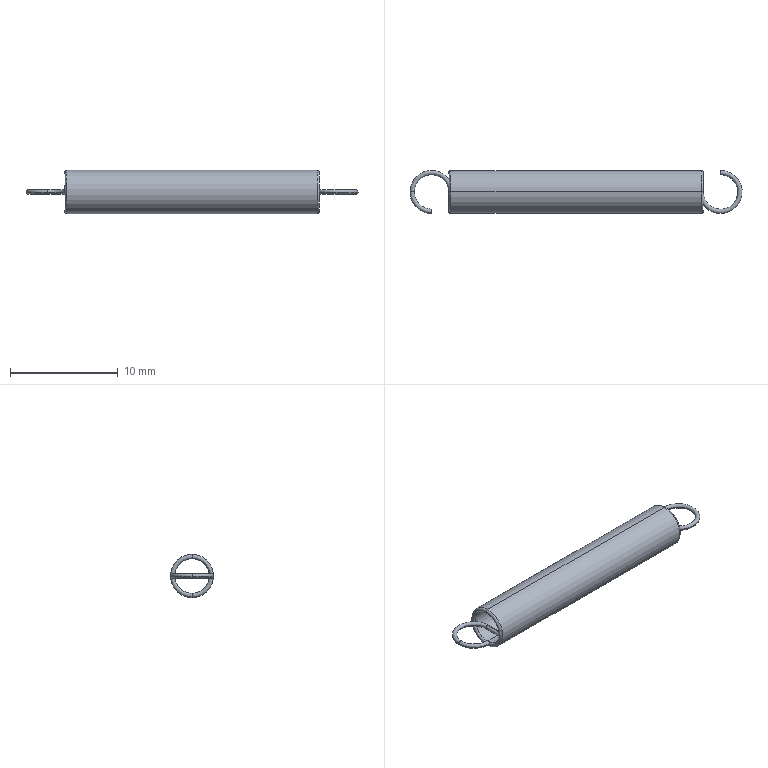Part | SolidWorks | features Revolution 5, RefAxis 1 | 1 solid | 20 faces | box 30.8 x 4 x 4 mm | volume 108.92 mm3 | torus 10 | cylinder 8 | plane 2 | commonest cylinder face diameters 0.4 x4 3.2 x2 4 x2
STEP:
#1=CARTESIAN_POINT('',(-0.4,0.,0.));
#2=VERTEX_POINT('',#1);
#3=CARTESIAN_POINT('',(0.,0.,0.));
#4=VERTEX_POINT('',#3);
#5=CARTESIAN_POINT('',(-0.2,0.,0.));
#6=DIRECTION('',(0.,-1.,0.));
#7=DIRECTION('',(0.,0.,-1.));
#8=AXIS2_PLACEMENT_3D('',#5,#6,#7);
#9=CIRCLE('',#8,0.2);
#10=EDGE_CURVE('',#2,#4,#9,.T.);
#11=ORIENTED_EDGE('',*,*,#10,.F.);
#12=CARTESIAN_POINT('',(3.6,0.,0.));
#13=VERTEX_POINT('',#12);
#14=CARTESIAN_POINT('',(1.6,0.,0.));
#15=DIRECTION('',(0.,0.,-1.));
#16=DIRECTION('',(-1.,0.,0.));
#17=AXIS2_PLACEMENT_3D('',#14,#15,#16);
#18=CIRCLE('',#17,2.);
#19=EDGE_CURVE('',#2,#13,#18,.T.);
#20=ORIENTED_EDGE('',*,*,#19,.T.);
#21=CARTESIAN_POINT('',(3.4,0.,-0.2));
#22=VERTEX_POINT('',#21);
#23=CARTESIAN_POINT('',(3.4,0.,0.));
#24=DIRECTION('',(0.,-1.,0.));
#25=DIRECTION('',(0.,0.,-1.));
#26=AXIS2_PLACEMENT_3D('',#23,#24,#25);
#27=CIRCLE('',#26,0.2);
#28=EDGE_CURVE('',#22,#13,#27,.T.);
#29=ORIENTED_EDGE('',*,*,#28,.F.);
#30=CARTESIAN_POINT('',(3.2,0.,0.));
#31=VERTEX_POINT('',#30);
#32=CARTESIAN_POINT('',(3.4,0.,0.));
#33=DIRECTION('',(0.,-1.,0.));
#34=DIRECTION('',(0.,0.,-1.));
#35=AXIS2_PLACEMENT_3D('',#32,#33,#34);
#36=CIRCLE('',#35,0.2);
#37=EDGE_CURVE('',#31,#22,#36,.T.);
#38=ORIENTED_EDGE('',*,*,#37,.F.);
#39=CARTESIAN_POINT('',(1.6,0.,0.));
#40=DIRECTION('',(0.,0.,-1.));
#41=DIRECTION('',(-1.,0.,0.));
#42=AXIS2_PLACEMENT_3D('',#39,#40,#41);
#43=CIRCLE('',#42,1.6);
#44=EDGE_CURVE('',#4,#31,#43,.T.);
#45=ORIENTED_EDGE('',*,*,#44,.F.);
#46=EDGE_LOOP('',(#11,#20,#29,#38,#45));
#47=FACE_OUTER_BOUND('',#46,.T.);
#48=CARTESIAN_POINT('',(1.6,0.,0.));
#49=DIRECTION('',(0.,0.,-1.));
#50=DIRECTION('',(-1.,0.,0.));
#51=AXIS2_PLACEMENT_3D('',#48,#49,#50);
#52=TOROIDAL_SURFACE('',#51,1.8,0.2);
#53=ADVANCED_FACE('',(#47),#52,.T.);
#54=CARTESIAN_POINT('',(28.372,1.6,0.));
#55=VERTEX_POINT('',#54);
#56=CARTESIAN_POINT('',(28.365,2.,0.));
#57=VERTEX_POINT('',#56);
#58=CARTESIAN_POINT('',(28.369,1.8,0.));
#59=DIRECTION('',(0.9998,0.01745,0.));
#60=DIRECTION('',(0.,0.,1.));
#61=AXIS2_PLACEMENT_3D('',#58,#59,#60);
#62=CIRCLE('',#61,0.2);
#63=EDGE_CURVE('',#55,#57,#62,.T.);
#64=ORIENTED_EDGE('',*,*,#63,.T.);
#65=CARTESIAN_POINT('',(26.4,0.,0.));
#66=VERTEX_POINT('',#65);
#67=CARTESIAN_POINT('',(28.4,0.,0.));
#68=DIRECTION('',(0.,0.,-1.));
#69=DIRECTION('',(-1.,0.,0.));
#70=AXIS2_PLACEMENT_3D('',#67,#68,#69);
#71=CIRCLE('',#70,2.);
#72=EDGE_CURVE('',#57,#66,#71,.T.);
#73=ORIENTED_EDGE('',*,*,#72,.T.);
#74=CARTESIAN_POINT('',(26.6,0.,-0.2));
#75=VERTEX_POINT('',#74);
#76=CARTESIAN_POINT('',(26.6,0.,0.));
#77=DIRECTION('',(0.,1.,0.));
#78=DIRECTION('',(0.,0.,1.));
#79=AXIS2_PLACEMENT_3D('',#76,#77,#78);
#80=CIRCLE('',#79,0.2);
#81=EDGE_CURVE('',#75,#66,#80,.T.);
#82=ORIENTED_EDGE('',*,*,#81,.F.);
#83=CARTESIAN_POINT('',(26.8,0.,0.));
#84=VERTEX_POINT('',#83);
#85=CARTESIAN_POINT('',(26.6,0.,0.));
#86=DIRECTION('',(0.,1.,0.));
#87=DIRECTION('',(0.,0.,1.));
#88=AXIS2_PLACEMENT_3D('',#85,#86,#87);
#89=CIRCLE('',#88,0.2);
#90=EDGE_CURVE('',#84,#75,#89,.T.);
#91=ORIENTED_EDGE('',*,*,#90,.F.);
#92=CARTESIAN_POINT('',(28.4,0.,0.));
#93=DIRECTION('',(0.,0.,-1.));
#94=DIRECTION('',(-1.,0.,0.));
#95=AXIS2_PLACEMENT_3D('',#92,#93,#94);
#96=CIRCLE('',#95,1.6);
#97=EDGE_CURVE('',#55,#84,#96,.T.);
#98=ORIENTED_EDGE('',*,*,#97,.F.);
#99=EDGE_LOOP('',(#64,#73,#82,#91,#98));
#100=FACE_OUTER_BOUND('',#99,.T.);
#101=CARTESIAN_POINT('',(28.4,0.,0.));
#102=DIRECTION('',(0.,0.,-1.));
#103=DIRECTION('',(-1.,0.,0.));
#104=AXIS2_PLACEMENT_3D('',#101,#102,#103);
#105=TOROIDAL_SURFACE('',#104,1.8,0.2);
#106=ADVANCED_FACE('',(#100),#105,.T.);
#107=CARTESIAN_POINT('',(1.635,-2.,0.));
#108=VERTEX_POINT('',#107);
#109=CARTESIAN_POINT('',(1.628,-1.6,0.));
#110=VERTEX_POINT('',#109);
#111=CARTESIAN_POINT('',(1.631,-1.8,0.));
#112=DIRECTION('',(0.9998,0.01745,0.));
#113=DIRECTION('',(0.,0.,1.));
#114=AXIS2_PLACEMENT_3D('',#111,#112,#113);
#115=CIRCLE('',#114,0.2);
#116=EDGE_CURVE('',#108,#110,#115,.T.);
#117=ORIENTED_EDGE('',*,*,#116,.F.);
#118=CARTESIAN_POINT('',(1.6,0.,0.));
#119=DIRECTION('',(0.,0.,-1.));
#120=DIRECTION('',(-1.,0.,0.));
#121=AXIS2_PLACEMENT_3D('',#118,#119,#120);
#122=CIRCLE('',#121,2.);
#123=EDGE_CURVE('',#108,#2,#122,.T.);
#124=ORIENTED_EDGE('',*,*,#123,.T.);
#125=ORIENTED_EDGE('',*,*,#10,.T.);
#126=CARTESIAN_POINT('',(1.6,0.,0.));
#127=DIRECTION('',(0.,0.,-1.));
#128=DIRECTION('',(-1.,0.,0.));
#129=AXIS2_PLACEMENT_3D('',#126,#127,#128);
#130=CIRCLE('',#129,1.6);
#131=EDGE_CURVE('',#110,#4,#130,.T.);
#132=ORIENTED_EDGE('',*,*,#131,.F.);
#133=EDGE_LOOP('',(#117,#124,#125,#132));
#134=FACE_OUTER_BOUND('',#133,.T.);
#135=CARTESIAN_POINT('',(1.6,0.,0.));
#136=DIRECTION('',(0.,0.,-1.));
#137=DIRECTION('',(-1.,0.,0.));
#138=AXIS2_PLACEMENT_3D('',#135,#136,#137);
#139=TOROIDAL_SURFACE('',#138,1.8,0.2);
#140=ADVANCED_FACE('',(#134),#139,.T.);
#141=ORIENTED_EDGE('',*,*,#123,.F.);
#142=CARTESIAN_POINT('',(1.631,-1.8,0.));
#143=DIRECTION('',(0.9998,0.01745,0.));
#144=DIRECTION('',(0.,0.,1.));
#145=AXIS2_PLACEMENT_3D('',#142,#143,#144);
#146=CIRCLE('',#145,0.2);
#147=EDGE_CURVE('',#110,#108,#146,.T.);
#148=ORIENTED_EDGE('',*,*,#147,.F.);
#149=ORIENTED_EDGE('',*,*,#131,.T.);
#150=CARTESIAN_POINT('',(-0.2,0.,0.));
#151=DIRECTION('',(0.,-1.,0.));
#152=DIRECTION('',(0.,0.,-1.));
#153=AXIS2_PLACEMENT_3D('',#150,#151,#152);
#154=CIRCLE('',#153,0.2);
#155=EDGE_CURVE('',#4,#2,#154,.T.);
#156=ORIENTED_EDGE('',*,*,#155,.T.);
#157=EDGE_LOOP('',(#141,#148,#149,#156));
#158=FACE_OUTER_BOUND('',#157,.T.);
#159=CARTESIAN_POINT('',(1.6,0.,0.));
#160=DIRECTION('',(0.,0.,-1.));
#161=DIRECTION('',(-1.,0.,0.));
#162=AXIS2_PLACEMENT_3D('',#159,#160,#161);
#163=TOROIDAL_SURFACE('',#162,1.8,0.2);
#164=ADVANCED_FACE('',(#158),#163,.T.);
#165=ORIENTED_EDGE('',*,*,#28,.T.);
#166=CARTESIAN_POINT('',(3.4,0.,0.2));
#167=VERTEX_POINT('',#166);
#168=CARTESIAN_POINT('',(3.4,0.,0.));
#169=DIRECTION('',(0.,-1.,0.));
#170=DIRECTION('',(0.,0.,-1.));
#171=AXIS2_PLACEMENT_3D('',#168,#169,#170);
#172=CIRCLE('',#171,0.2);
#173=EDGE_CURVE('',#13,#167,#172,.T.);
#174=ORIENTED_EDGE('',*,*,#173,.T.);
#175=CARTESIAN_POINT('',(3.4,-1.587,0.2));
#176=VERTEX_POINT('',#175);
#177=CARTESIAN_POINT('',(3.4,-1.8,0.2));
#178=DIRECTION('',(0.,-1.,0.));
#179=VECTOR('',#178,1000.);
#180=LINE('',#177,#179);
#181=EDGE_CURVE('',#167,#176,#180,.T.);
#182=ORIENTED_EDGE('',*,*,#181,.T.);
#183=CARTESIAN_POINT('',(3.4,-1.587,-0.2));
#184=VERTEX_POINT('',#183);
#185=CARTESIAN_POINT('',(3.4,-1.587,-0.2));
#186=CARTESIAN_POINT('',(3.453,-1.587,-0.2));
#187=CARTESIAN_POINT('',(3.505,-1.59,-0.1783));
#188=CARTESIAN_POINT('',(3.578,-1.597,-0.1045));
#189=CARTESIAN_POINT('',(3.6,-1.6,-0.05231));
#190=CARTESIAN_POINT('',(3.6,-1.6,0.05216));
#191=CARTESIAN_POINT('',(3.579,-1.597,0.1041));
#192=CARTESIAN_POINT('',(3.504,-1.59,0.1787));
#193=CARTESIAN_POINT('',(3.452,-1.587,0.2));
#194=CARTESIAN_POINT('',(3.4,-1.587,0.2));
#195=B_SPLINE_CURVE_WITH_KNOTS('',3,(#185,#186,#187,#188,#189,#190,#191,#192,#193,#194),.UNSPECIFIED.,.F.,.F.,(4,2,2,2,4),(0.,0.0001565,0.000313,0.0004694,0.0006259),.UNSPECIFIED.);
#196=EDGE_CURVE('',#184,#176,#195,.T.);
#197=ORIENTED_EDGE('',*,*,#196,.F.);
#198=CARTESIAN_POINT('',(3.4,-1.8,-0.2));
#199=DIRECTION('',(0.,-1.,0.));
#200=VECTOR('',#199,1000.);
#201=LINE('',#198,#200);
#202=EDGE_CURVE('',#22,#184,#201,.T.);
#203=ORIENTED_EDGE('',*,*,#202,.F.);
#204=EDGE_LOOP('',(#165,#174,#182,#197,#203));
#205=FACE_OUTER_BOUND('',#204,.T.);
#206=CARTESIAN_POINT('',(3.4,-1.8,0.));
#207=DIRECTION('',(0.,-1.,0.));
#208=DIRECTION('',(0.,0.,-1.));
#209=AXIS2_PLACEMENT_3D('',#206,#207,#208);
#210=CYLINDRICAL_SURFACE('',#209,0.2);
#211=ADVANCED_FACE('',(#205),#210,.T.);
#212=CARTESIAN_POINT('',(26.6,0.,0.2));
#213=VERTEX_POINT('',#212);
#214=CARTESIAN_POINT('',(26.6,0.,0.));
#215=DIRECTION('',(0.,1.,0.));
#216=DIRECTION('',(0.,0.,1.));
#217=AXIS2_PLACEMENT_3D('',#214,#215,#216);
#218=CIRCLE('',#217,0.2);
#219=EDGE_CURVE('',#213,#84,#218,.T.);
#220=ORIENTED_EDGE('',*,*,#219,.T.);
#221=ORIENTED_EDGE('',*,*,#90,.T.);
#222=CARTESIAN_POINT('',(26.6,1.587,-0.2));
#223=VERTEX_POINT('',#222);
#224=CARTESIAN_POINT('',(26.6,0.,-0.2));
#225=DIRECTION('',(0.,1.,0.));
#226=VECTOR('',#225,1000.);
#227=LINE('',#224,#226);
#228=EDGE_CURVE('',#75,#223,#227,.T.);
#229=ORIENTED_EDGE('',*,*,#228,.T.);
#230=CARTESIAN_POINT('',(26.8,1.8,0.));
#231=VERTEX_POINT('',#230);
#232=CARTESIAN_POINT('',(26.6,1.587,-0.2));
#233=CARTESIAN_POINT('',(26.633,1.587,-0.2));
#234=CARTESIAN_POINT('',(26.664,1.597,-0.1917));
#235=CARTESIAN_POINT('',(26.716,1.626,-0.1654));
#236=CARTESIAN_POINT('',(26.737,1.645,-0.1481));
#237=CARTESIAN_POINT('',(26.785,1.707,-0.09082));
#238=CARTESIAN_POINT('',(26.8,1.754,-0.04562));
#239=CARTESIAN_POINT('',(26.8,1.8,0.));
#240=B_SPLINE_CURVE_WITH_KNOTS('',3,(#232,#233,#234,#235,#236,#237,#238,#239),.UNSPECIFIED.,.F.,.F.,(4,2,2,4),(0.000000196,0.000097,0.0001938,0.0003874),.UNSPECIFIED.);
#241=EDGE_CURVE('',#223,#231,#240,.T.);
#242=ORIENTED_EDGE('',*,*,#241,.T.);
#243=CARTESIAN_POINT('',(26.6,1.587,0.2));
#244=VERTEX_POINT('',#243);
#245=CARTESIAN_POINT('',(26.8,1.8,0.));
#246=CARTESIAN_POINT('',(26.8,1.755,0.04539));
#247=CARTESIAN_POINT('',(26.785,1.707,0.09079));
#248=CARTESIAN_POINT('',(26.737,1.646,0.1479));
#249=CARTESIAN_POINT('',(26.716,1.626,0.1653));
#250=CARTESIAN_POINT('',(26.664,1.597,0.1916));
#251=CARTESIAN_POINT('',(26.633,1.587,0.2));
#252=CARTESIAN_POINT('',(26.6,1.587,0.2));
#253=B_SPLINE_CURVE_WITH_KNOTS('',3,(#245,#246,#247,#248,#249,#250,#251,#252),.UNSPECIFIED.,.F.,.F.,(4,2,2,4),(-0.000002828,0.0001898,0.0002861,0.0003825),.UNSPECIFIED.);
#254=EDGE_CURVE('',#231,#244,#253,.T.);
#255=ORIENTED_EDGE('',*,*,#254,.T.);
#256=CARTESIAN_POINT('',(26.6,0.,0.2));
#257=DIRECTION('',(0.,1.,0.));
#258=VECTOR('',#257,1000.);
#259=LINE('',#256,#258);
#260=EDGE_CURVE('',#213,#244,#259,.T.);
#261=ORIENTED_EDGE('',*,*,#260,.F.);
#262=EDGE_LOOP('',(#220,#221,#229,#242,#255,#261));
#263=FACE_OUTER_BOUND('',#262,.T.);
#264=CARTESIAN_POINT('',(26.6,0.,0.));
#265=DIRECTION('',(0.,1.,0.));
#266=DIRECTION('',(0.,0.,1.));
#267=AXIS2_PLACEMENT_3D('',#264,#265,#266);
#268=CYLINDRICAL_SURFACE('',#267,0.2);
#269=ADVANCED_FACE('',(#263),#268,.T.);
#270=CARTESIAN_POINT('',(26.6,0.,2.));
#271=VERTEX_POINT('',#270);
#272=CARTESIAN_POINT('',(26.6,0.,-2.));
#273=VERTEX_POINT('',#272);
#274=CARTESIAN_POINT('',(26.6,0.,0.));
#275=DIRECTION('',(-1.,0.,0.));
#276=DIRECTION('',(0.,0.,1.));
#277=AXIS2_PLACEMENT_3D('',#274,#275,#276);
#278=CIRCLE('',#277,2.);
#279=EDGE_CURVE('',#271,#273,#278,.T.);
#280=ORIENTED_EDGE('',*,*,#279,.T.);
#281=CARTESIAN_POINT('',(3.4,0.,-2.));
#282=VERTEX_POINT('',#281);
#283=CARTESIAN_POINT('',(26.8,0.,-2.));
#284=DIRECTION('',(-1.,0.,0.));
#285=VECTOR('',#284,1000.);
#286=LINE('',#283,#285);
#287=EDGE_CURVE('',#273,#282,#286,.T.);
#288=ORIENTED_EDGE('',*,*,#287,.T.);
#289=CARTESIAN_POINT('',(3.4,0.,2.));
#290=VERTEX_POINT('',#289);
#291=CARTESIAN_POINT('',(3.4,0.,0.));
#292=DIRECTION('',(-1.,0.,0.));
#293=DIRECTION('',(0.,0.,1.));
#294=AXIS2_PLACEMENT_3D('',#291,#292,#293);
#295=CIRCLE('',#294,2.);
#296=EDGE_CURVE('',#290,#282,#295,.T.);
#297=ORIENTED_EDGE('',*,*,#296,.F.);
#298=CARTESIAN_POINT('',(26.8,0.,2.));
#299=DIRECTION('',(-1.,0.,0.));
#300=VECTOR('',#299,1000.);
#301=LINE('',#298,#300);
#302=EDGE_CURVE('',#271,#290,#301,.T.);
#303=ORIENTED_EDGE('',*,*,#302,.F.);
#304=EDGE_LOOP('',(#280,#288,#297,#303));
#305=FACE_OUTER_BOUND('',#304,.T.);
#306=CARTESIAN_POINT('',(26.8,0.,0.));
#307=DIRECTION('',(-1.,0.,0.));
#308=DIRECTION('',(0.,0.,1.));
#309=AXIS2_PLACEMENT_3D('',#306,#307,#308);
#310=CYLINDRICAL_SURFACE('',#309,2.);
#311=ADVANCED_FACE('',(#305),#310,.T.);
#312=ORIENTED_EDGE('',*,*,#296,.T.);
#313=CARTESIAN_POINT('',(3.4,0.,-1.6));
#314=VERTEX_POINT('',#313);
#315=CARTESIAN_POINT('',(3.4,0.,-1.8));
#316=DIRECTION('',(0.,1.,0.));
#317=DIRECTION('',(0.,0.,1.));
#318=AXIS2_PLACEMENT_3D('',#315,#316,#317);
#319=CIRCLE('',#318,0.2);
#320=EDGE_CURVE('',#282,#314,#319,.T.);
#321=ORIENTED_EDGE('',*,*,#320,.T.);
#322=CARTESIAN_POINT('',(3.4,0.,1.6));
#323=VERTEX_POINT('',#322);
#324=CARTESIAN_POINT('',(3.4,0.,0.));
#325=DIRECTION('',(-1.,0.,0.));
#326=DIRECTION('',(0.,0.,1.));
#327=AXIS2_PLACEMENT_3D('',#324,#325,#326);
#328=CIRCLE('',#327,1.6);
#329=EDGE_CURVE('',#323,#314,#328,.T.);
#330=ORIENTED_EDGE('',*,*,#329,.F.);
#331=CARTESIAN_POINT('',(3.4,0.,1.8));
#332=DIRECTION('',(0.,-1.,0.));
#333=DIRECTION('',(0.,0.,-1.));
#334=AXIS2_PLACEMENT_3D('',#331,#332,#333);
#335=CIRCLE('',#334,0.2);
#336=EDGE_CURVE('',#290,#323,#335,.T.);
#337=ORIENTED_EDGE('',*,*,#336,.F.);
#338=EDGE_LOOP('',(#312,#321,#330,#337));
#339=FACE_OUTER_BOUND('',#338,.T.);
#340=CARTESIAN_POINT('',(3.4,0.,0.));
#341=DIRECTION('',(-1.,0.,0.));
#342=DIRECTION('',(0.,0.,1.));
#343=AXIS2_PLACEMENT_3D('',#340,#341,#342);
#344=TOROIDAL_SURFACE('',#343,1.8,0.2);
#345=ADVANCED_FACE('',(#339),#344,.T.);
#346=CARTESIAN_POINT('',(26.6,0.,-1.6));
#347=VERTEX_POINT('',#346);
#348=CARTESIAN_POINT('',(26.6,0.,0.));
#349=DIRECTION('',(-1.,0.,0.));
#350=DIRECTION('',(0.,0.,1.));
#351=AXIS2_PLACEMENT_3D('',#348,#349,#350);
#352=CIRCLE('',#351,1.6);
#353=EDGE_CURVE('',#223,#347,#352,.T.);
#354=ORIENTED_EDGE('',*,*,#353,.T.);
#355=CARTESIAN_POINT('',(26.6,0.,-1.8));
#356=DIRECTION('',(0.,1.,0.));
#357=DIRECTION('',(0.,0.,1.));
#358=AXIS2_PLACEMENT_3D('',#355,#356,#357);
#359=CIRCLE('',#358,0.2);
#360=EDGE_CURVE('',#347,#273,#359,.T.);
#361=ORIENTED_EDGE('',*,*,#360,.T.);
#362=ORIENTED_EDGE('',*,*,#279,.F.);
#363=CARTESIAN_POINT('',(26.6,0.,1.6));
#364=VERTEX_POINT('',#363);
#365=CARTESIAN_POINT('',(26.6,0.,1.8));
#366=DIRECTION('',(0.,-1.,0.));
#367=DIRECTION('',(0.,0.,-1.));
#368=AXIS2_PLACEMENT_3D('',#365,#366,#367);
#369=CIRCLE('',#368,0.2);
#370=EDGE_CURVE('',#364,#271,#369,.T.);
#371=ORIENTED_EDGE('',*,*,#370,.F.);
#372=CARTESIAN_POINT('',(26.6,0.,0.));
#373=DIRECTION('',(-1.,0.,0.));
#374=DIRECTION('',(0.,0.,1.));
#375=AXIS2_PLACEMENT_3D('',#372,#373,#374);
#376=CIRCLE('',#375,1.6);
#377=EDGE_CURVE('',#364,#244,#376,.T.);
#378=ORIENTED_EDGE('',*,*,#377,.T.);
#379=ORIENTED_EDGE('',*,*,#254,.F.);
#380=ORIENTED_EDGE('',*,*,#241,.F.);
#381=EDGE_LOOP('',(#354,#361,#362,#371,#378,#379,#380));
#382=FACE_OUTER_BOUND('',#381,.T.);
#383=CARTESIAN_POINT('',(26.6,0.,0.));
#384=DIRECTION('',(-1.,0.,0.));
#385=DIRECTION('',(0.,0.,1.));
#386=AXIS2_PLACEMENT_3D('',#383,#384,#385);
#387=TOROIDAL_SURFACE('',#386,1.8,0.2);
#388=ADVANCED_FACE('',(#382),#387,.T.);
#389=CARTESIAN_POINT('',(26.6,0.,0.));
#390=DIRECTION('',(-1.,0.,0.));
#391=DIRECTION('',(0.,0.,1.));
#392=AXIS2_PLACEMENT_3D('',#389,#390,#391);
#393=CIRCLE('',#392,1.6);
#394=EDGE_CURVE('',#347,#364,#393,.T.);
#395=ORIENTED_EDGE('',*,*,#394,.F.);
#396=CARTESIAN_POINT('',(26.8,0.,-1.6));
#397=DIRECTION('',(-1.,0.,0.));
#398=VECTOR('',#397,1000.);
#399=LINE('',#396,#398);
#400=EDGE_CURVE('',#347,#314,#399,.T.);
#401=ORIENTED_EDGE('',*,*,#400,.T.);
#402=CARTESIAN_POINT('',(3.4,0.,0.));
#403=DIRECTION('',(-1.,0.,0.));
#404=DIRECTION('',(0.,0.,1.));
#405=AXIS2_PLACEMENT_3D('',#402,#403,#404);
#406=CIRCLE('',#405,1.6);
#407=EDGE_CURVE('',#314,#184,#406,.T.);
#408=ORIENTED_EDGE('',*,*,#407,.T.);
#409=ORIENTED_EDGE('',*,*,#196,.T.);
#410=CARTESIAN_POINT('',(3.4,0.,0.));
#411=DIRECTION('',(-1.,0.,0.));
#412=DIRECTION('',(0.,0.,1.));
#413=AXIS2_PLACEMENT_3D('',#410,#411,#412);
#414=CIRCLE('',#413,1.6);
#415=EDGE_CURVE('',#176,#323,#414,.T.);
#416=ORIENTED_EDGE('',*,*,#415,.T.);
#417=CARTESIAN_POINT('',(26.8,0.,1.6));
#418=DIRECTION('',(-1.,0.,0.));
#419=VECTOR('',#418,1000.);
#420=LINE('',#417,#419);
#421=EDGE_CURVE('',#364,#323,#420,.T.);
#422=ORIENTED_EDGE('',*,*,#421,.F.);
#423=EDGE_LOOP('',(#395,#401,#408,#409,#416,#422));
#424=FACE_OUTER_BOUND('',#423,.T.);
#425=CARTESIAN_POINT('',(26.8,0.,0.));
#426=DIRECTION('',(-1.,0.,0.));
#427=DIRECTION('',(0.,0.,1.));
#428=AXIS2_PLACEMENT_3D('',#425,#426,#427);
#429=CYLINDRICAL_SURFACE('',#428,1.6);
#430=ADVANCED_FACE('',(#424),#429,.F.);
#431=ORIENTED_EDGE('',*,*,#400,.F.);
#432=ORIENTED_EDGE('',*,*,#353,.F.);
#433=CARTESIAN_POINT('',(26.6,1.587,0.2));
#434=CARTESIAN_POINT('',(26.547,1.587,0.2));
#435=CARTESIAN_POINT('',(26.495,1.59,0.1783));
#436=CARTESIAN_POINT('',(26.422,1.597,0.1045));
#437=CARTESIAN_POINT('',(26.4,1.6,0.05231));
#438=CARTESIAN_POINT('',(26.4,1.6,-0.05216));
#439=CARTESIAN_POINT('',(26.421,1.597,-0.1041));
#440=CARTESIAN_POINT('',(26.496,1.59,-0.1787));
#441=CARTESIAN_POINT('',(26.548,1.587,-0.2));
#442=CARTESIAN_POINT('',(26.6,1.587,-0.2));
#443=B_SPLINE_CURVE_WITH_KNOTS('',3,(#433,#434,#435,#436,#437,#438,#439,#440,#441,#442),.UNSPECIFIED.,.F.,.F.,(4,2,2,2,4),(0.,0.0001565,0.000313,0.0004694,0.0006259),.UNSPECIFIED.);
#444=EDGE_CURVE('',#244,#223,#443,.T.);
#445=ORIENTED_EDGE('',*,*,#444,.F.);
#446=ORIENTED_EDGE('',*,*,#377,.F.);
#447=ORIENTED_EDGE('',*,*,#421,.T.);
#448=ORIENTED_EDGE('',*,*,#329,.T.);
#449=EDGE_LOOP('',(#431,#432,#445,#446,#447,#448));
#450=FACE_OUTER_BOUND('',#449,.T.);
#451=CARTESIAN_POINT('',(26.8,0.,0.));
#452=DIRECTION('',(-1.,0.,0.));
#453=DIRECTION('',(0.,0.,1.));
#454=AXIS2_PLACEMENT_3D('',#451,#452,#453);
#455=CYLINDRICAL_SURFACE('',#454,1.6);
#456=ADVANCED_FACE('',(#450),#455,.F.);
#457=ORIENTED_EDGE('',*,*,#360,.F.);
#458=ORIENTED_EDGE('',*,*,#394,.T.);
#459=ORIENTED_EDGE('',*,*,#370,.T.);
#460=CARTESIAN_POINT('',(26.6,0.,0.));
#461=DIRECTION('',(-1.,0.,0.));
#462=DIRECTION('',(0.,0.,1.));
#463=AXIS2_PLACEMENT_3D('',#460,#461,#462);
#464=CIRCLE('',#463,2.);
#465=EDGE_CURVE('',#273,#271,#464,.T.);
#466=ORIENTED_EDGE('',*,*,#465,.F.);
#467=EDGE_LOOP('',(#457,#458,#459,#466));
#468=FACE_OUTER_BOUND('',#467,.T.);
#469=CARTESIAN_POINT('',(26.6,0.,0.));
#470=DIRECTION('',(-1.,0.,0.));
#471=DIRECTION('',(0.,0.,1.));
#472=AXIS2_PLACEMENT_3D('',#469,#470,#471);
#473=TOROIDAL_SURFACE('',#472,1.8,0.2);
#474=ADVANCED_FACE('',(#468),#473,.T.);
#475=ORIENTED_EDGE('',*,*,#320,.F.);
#476=CARTESIAN_POINT('',(3.4,0.,0.));
#477=DIRECTION('',(-1.,0.,0.));
#478=DIRECTION('',(0.,0.,1.));
#479=AXIS2_PLACEMENT_3D('',#476,#477,#478);
#480=CIRCLE('',#479,2.);
#481=EDGE_CURVE('',#282,#290,#480,.T.);
#482=ORIENTED_EDGE('',*,*,#481,.T.);
#483=ORIENTED_EDGE('',*,*,#336,.T.);
#484=ORIENTED_EDGE('',*,*,#415,.F.);
#485=CARTESIAN_POINT('',(3.2,-1.8,0.));
#486=VERTEX_POINT('',#485);
#487=CARTESIAN_POINT('',(3.4,-1.587,0.2));
#488=CARTESIAN_POINT('',(3.367,-1.587,0.2));
#489=CARTESIAN_POINT('',(3.336,-1.597,0.1917));
#490=CARTESIAN_POINT('',(3.284,-1.626,0.1654));
#491=CARTESIAN_POINT('',(3.263,-1.645,0.1481));
#492=CARTESIAN_POINT('',(3.215,-1.707,0.09082));
#493=CARTESIAN_POINT('',(3.2,-1.754,0.04562));
#494=CARTESIAN_POINT('',(3.2,-1.8,0.));
#495=B_SPLINE_CURVE_WITH_KNOTS('',3,(#487,#488,#489,#490,#491,#492,#493,#494),.UNSPECIFIED.,.F.,.F.,(4,2,2,4),(0.000000196,0.000097,0.0001938,0.0003874),.UNSPECIFIED.);
#496=EDGE_CURVE('',#176,#486,#495,.T.);
#497=ORIENTED_EDGE('',*,*,#496,.T.);
#498=CARTESIAN_POINT('',(3.2,-1.8,0.));
#499=CARTESIAN_POINT('',(3.2,-1.755,-0.04539));
#500=CARTESIAN_POINT('',(3.215,-1.707,-0.09079));
#501=CARTESIAN_POINT('',(3.263,-1.646,-0.1479));
#502=CARTESIAN_POINT('',(3.284,-1.626,-0.1653));
#503=CARTESIAN_POINT('',(3.336,-1.597,-0.1916));
#504=CARTESIAN_POINT('',(3.367,-1.587,-0.2));
#505=CARTESIAN_POINT('',(3.4,-1.587,-0.2));
#506=B_SPLINE_CURVE_WITH_KNOTS('',3,(#498,#499,#500,#501,#502,#503,#504,#505),.UNSPECIFIED.,.F.,.F.,(4,2,2,4),(-0.000002828,0.0001898,0.0002861,0.0003825),.UNSPECIFIED.);
#507=EDGE_CURVE('',#486,#184,#506,.T.);
#508=ORIENTED_EDGE('',*,*,#507,.T.);
#509=ORIENTED_EDGE('',*,*,#407,.F.);
#510=EDGE_LOOP('',(#475,#482,#483,#484,#497,#508,#509));
#511=FACE_OUTER_BOUND('',#510,.T.);
#512=CARTESIAN_POINT('',(3.4,0.,0.));
#513=DIRECTION('',(-1.,0.,0.));
#514=DIRECTION('',(0.,0.,1.));
#515=AXIS2_PLACEMENT_3D('',#512,#513,#514);
#516=TOROIDAL_SURFACE('',#515,1.8,0.2);
#517=ADVANCED_FACE('',(#511),#516,.T.);
#518=ORIENTED_EDGE('',*,*,#287,.F.);
#519=ORIENTED_EDGE('',*,*,#465,.T.);
#520=ORIENTED_EDGE('',*,*,#302,.T.);
#521=ORIENTED_EDGE('',*,*,#481,.F.);
#522=EDGE_LOOP('',(#518,#519,#520,#521));
#523=FACE_OUTER_BOUND('',#522,.T.);
#524=CARTESIAN_POINT('',(26.8,0.,0.));
#525=DIRECTION('',(-1.,0.,0.));
#526=DIRECTION('',(0.,0.,1.));
#527=AXIS2_PLACEMENT_3D('',#524,#525,#526);
#528=CYLINDRICAL_SURFACE('',#527,2.);
#529=ADVANCED_FACE('',(#523),#528,.T.);
#530=ORIENTED_EDGE('',*,*,#228,.F.);
#531=ORIENTED_EDGE('',*,*,#81,.T.);
#532=CARTESIAN_POINT('',(26.6,0.,0.));
#533=DIRECTION('',(0.,1.,0.));
#534=DIRECTION('',(0.,0.,1.));
#535=AXIS2_PLACEMENT_3D('',#532,#533,#534);
#536=CIRCLE('',#535,0.2);
#537=EDGE_CURVE('',#66,#213,#536,.T.);
#538=ORIENTED_EDGE('',*,*,#537,.T.);
#539=ORIENTED_EDGE('',*,*,#260,.T.);
#540=ORIENTED_EDGE('',*,*,#444,.T.);
#541=EDGE_LOOP('',(#530,#531,#538,#539,#540));
#542=FACE_OUTER_BOUND('',#541,.T.);
#543=CARTESIAN_POINT('',(26.6,0.,0.));
#544=DIRECTION('',(0.,1.,0.));
#545=DIRECTION('',(0.,0.,1.));
#546=AXIS2_PLACEMENT_3D('',#543,#544,#545);
#547=CYLINDRICAL_SURFACE('',#546,0.2);
#548=ADVANCED_FACE('',(#542),#547,.T.);
#549=ORIENTED_EDGE('',*,*,#72,.F.);
#550=CARTESIAN_POINT('',(28.369,1.8,0.));
#551=DIRECTION('',(0.9998,0.01745,0.));
#552=DIRECTION('',(0.,0.,1.));
#553=AXIS2_PLACEMENT_3D('',#550,#551,#552);
#554=CIRCLE('',#553,0.2);
#555=EDGE_CURVE('',#57,#55,#554,.T.);
#556=ORIENTED_EDGE('',*,*,#555,.T.);
#557=ORIENTED_EDGE('',*,*,#97,.T.);
#558=ORIENTED_EDGE('',*,*,#219,.F.);
#559=ORIENTED_EDGE('',*,*,#537,.F.);
#560=EDGE_LOOP('',(#549,#556,#557,#558,#559));
#561=FACE_OUTER_BOUND('',#560,.T.);
#562=CARTESIAN_POINT('',(28.4,0.,0.));
#563=DIRECTION('',(0.,0.,-1.));
#564=DIRECTION('',(-1.,0.,0.));
#565=AXIS2_PLACEMENT_3D('',#562,#563,#564);
#566=TOROIDAL_SURFACE('',#565,1.8,0.2);
#567=ADVANCED_FACE('',(#561),#566,.T.);
#568=ORIENTED_EDGE('',*,*,#63,.F.);
#569=ORIENTED_EDGE('',*,*,#555,.F.);
#570=EDGE_LOOP('',(#568,#569));
#571=FACE_OUTER_BOUND('',#570,.T.);
#572=CARTESIAN_POINT('',(28.369,1.8,0.));
#573=DIRECTION('',(0.9998,0.01745,0.));
#574=DIRECTION('',(0.,0.,1.));
#575=AXIS2_PLACEMENT_3D('',#572,#573,#574);
#576=PLANE('',#575);
#577=ADVANCED_FACE('',(#571),#576,.F.);
#578=ORIENTED_EDGE('',*,*,#181,.F.);
#579=CARTESIAN_POINT('',(3.4,0.,0.));
#580=DIRECTION('',(0.,-1.,0.));
#581=DIRECTION('',(0.,0.,-1.));
#582=AXIS2_PLACEMENT_3D('',#579,#580,#581);
#583=CIRCLE('',#582,0.2);
#584=EDGE_CURVE('',#167,#31,#583,.T.);
#585=ORIENTED_EDGE('',*,*,#584,.T.);
#586=ORIENTED_EDGE('',*,*,#37,.T.);
#587=ORIENTED_EDGE('',*,*,#202,.T.);
#588=ORIENTED_EDGE('',*,*,#507,.F.);
#589=ORIENTED_EDGE('',*,*,#496,.F.);
#590=EDGE_LOOP('',(#578,#585,#586,#587,#588,#589));
#591=FACE_OUTER_BOUND('',#590,.T.);
#592=CARTESIAN_POINT('',(3.4,-1.8,0.));
#593=DIRECTION('',(0.,-1.,0.));
#594=DIRECTION('',(0.,0.,-1.));
#595=AXIS2_PLACEMENT_3D('',#592,#593,#594);
#596=CYLINDRICAL_SURFACE('',#595,0.2);
#597=ADVANCED_FACE('',(#591),#596,.T.);
#598=ORIENTED_EDGE('',*,*,#19,.F.);
#599=ORIENTED_EDGE('',*,*,#155,.F.);
#600=ORIENTED_EDGE('',*,*,#44,.T.);
#601=ORIENTED_EDGE('',*,*,#584,.F.);
#602=ORIENTED_EDGE('',*,*,#173,.F.);
#603=EDGE_LOOP('',(#598,#599,#600,#601,#602));
#604=FACE_OUTER_BOUND('',#603,.T.);
#605=CARTESIAN_POINT('',(1.6,0.,0.));
#606=DIRECTION('',(0.,0.,-1.));
#607=DIRECTION('',(-1.,0.,0.));
#608=AXIS2_PLACEMENT_3D('',#605,#606,#607);
#609=TOROIDAL_SURFACE('',#608,1.8,0.2);
#610=ADVANCED_FACE('',(#604),#609,.T.);
#611=ORIENTED_EDGE('',*,*,#147,.T.);
#612=ORIENTED_EDGE('',*,*,#116,.T.);
#613=EDGE_LOOP('',(#611,#612));
#614=FACE_OUTER_BOUND('',#613,.T.);
#615=CARTESIAN_POINT('',(1.631,-1.8,0.));
#616=DIRECTION('',(0.9998,0.01745,0.));
#617=DIRECTION('',(0.,0.,1.));
#618=AXIS2_PLACEMENT_3D('',#615,#616,#617);
#619=PLANE('',#618);
#620=ADVANCED_FACE('',(#614),#619,.T.);
#621=CLOSED_SHELL('',(#53,#106,#140,#164,#211,#269,#311,#345,#388,#430,#456,#474,#517,#529,#548,#567,#577,#597,#610,#620));
#622=MANIFOLD_SOLID_BREP('',#621);
#623=CARTESIAN_POINT('',(0.,0.,0.));
#624=DIRECTION('',(0.,0.,1.));
#625=DIRECTION('',(1.,0.,0.));
#626=AXIS2_PLACEMENT_3D('',#623,#624,#625);
#627=(LENGTH_UNIT()NAMED_UNIT(*)SI_UNIT(.MILLI.,.METRE.));
#628=UNCERTAINTY_MEASURE_WITH_UNIT(LENGTH_MEASURE(0.00001),#627,'','');
#629=(NAMED_UNIT(*)PLANE_ANGLE_UNIT()SI_UNIT($,.RADIAN.));
#630=(NAMED_UNIT(*)SI_UNIT($,.STERADIAN.)SOLID_ANGLE_UNIT());
#631=(GEOMETRIC_REPRESENTATION_CONTEXT(3)GLOBAL_UNCERTAINTY_ASSIGNED_CONTEXT((#628))GLOBAL_UNIT_ASSIGNED_CONTEXT((#627,#629,#630))REPRESENTATION_CONTEXT('',''));
#632=ADVANCED_BREP_SHAPE_REPRESENTATION('',(#622,#626),#631);